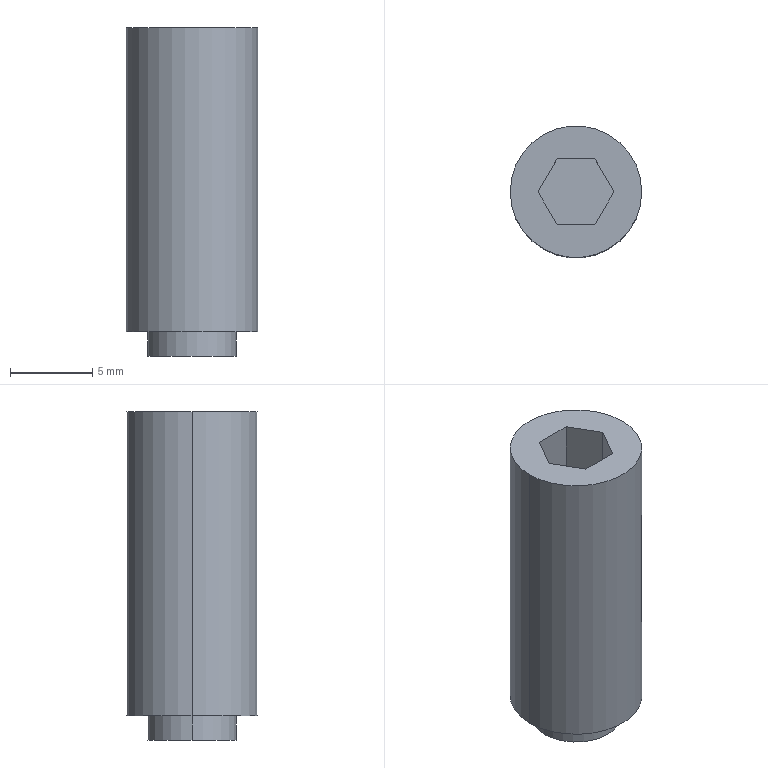Part | SolidWorks | features BaseBody 1 | 1 solid | 14 faces | box 8 x 8 x 20 mm | volume 908.839 mm3 | plane 10 | cylinder 4 | commonest cylinder face diameters 5.4 x2 8 x2
STEP:
#1=CARTESIAN_POINT('',(-2.7,0.,-1.5));
#2=VERTEX_POINT('',#1);
#3=CARTESIAN_POINT('',(2.7,0.,-1.5));
#4=VERTEX_POINT('',#3);
#5=CARTESIAN_POINT('',(0.,0.,-1.5));
#6=DIRECTION('',(0.,0.,-1.));
#7=DIRECTION('',(-1.,0.,0.));
#8=AXIS2_PLACEMENT_3D('',#5,#6,#7);
#9=CIRCLE('',#8,2.7);
#10=EDGE_CURVE('',#2,#4,#9,.T.);
#11=ORIENTED_EDGE('',*,*,#10,.T.);
#12=CARTESIAN_POINT('',(2.7,0.,-3.));
#13=VERTEX_POINT('',#12);
#14=CARTESIAN_POINT('',(2.7,0.,-3.));
#15=DIRECTION('',(0.,0.,-1.));
#16=VECTOR('',#15,1000.);
#17=LINE('',#14,#16);
#18=EDGE_CURVE('',#4,#13,#17,.T.);
#19=ORIENTED_EDGE('',*,*,#18,.T.);
#20=CARTESIAN_POINT('',(-2.7,0.,-3.));
#21=VERTEX_POINT('',#20);
#22=CARTESIAN_POINT('',(0.,0.,-3.));
#23=DIRECTION('',(0.,0.,-1.));
#24=DIRECTION('',(-1.,0.,0.));
#25=AXIS2_PLACEMENT_3D('',#22,#23,#24);
#26=CIRCLE('',#25,2.7);
#27=EDGE_CURVE('',#21,#13,#26,.T.);
#28=ORIENTED_EDGE('',*,*,#27,.F.);
#29=CARTESIAN_POINT('',(-2.7,0.,-3.));
#30=DIRECTION('',(0.,0.,-1.));
#31=VECTOR('',#30,1000.);
#32=LINE('',#29,#31);
#33=EDGE_CURVE('',#2,#21,#32,.T.);
#34=ORIENTED_EDGE('',*,*,#33,.F.);
#35=EDGE_LOOP('',(#11,#19,#28,#34));
#36=FACE_OUTER_BOUND('',#35,.T.);
#37=CARTESIAN_POINT('',(0.,0.,-3.));
#38=DIRECTION('',(0.,0.,-1.));
#39=DIRECTION('',(-1.,0.,0.));
#40=AXIS2_PLACEMENT_3D('',#37,#38,#39);
#41=CYLINDRICAL_SURFACE('',#40,2.7);
#42=ADVANCED_FACE('',(#36),#41,.T.);
#43=CARTESIAN_POINT('',(-4.,0.,17.));
#44=VERTEX_POINT('',#43);
#45=CARTESIAN_POINT('',(4.,0.,17.));
#46=VERTEX_POINT('',#45);
#47=CARTESIAN_POINT('',(0.,0.,17.));
#48=DIRECTION('',(0.,0.,-1.));
#49=DIRECTION('',(-1.,0.,0.));
#50=AXIS2_PLACEMENT_3D('',#47,#48,#49);
#51=CIRCLE('',#50,4.);
#52=EDGE_CURVE('',#44,#46,#51,.T.);
#53=ORIENTED_EDGE('',*,*,#52,.T.);
#54=CARTESIAN_POINT('',(4.,0.,-1.5));
#55=VERTEX_POINT('',#54);
#56=CARTESIAN_POINT('',(4.,0.,-3.));
#57=DIRECTION('',(0.,0.,-1.));
#58=VECTOR('',#57,1000.);
#59=LINE('',#56,#58);
#60=EDGE_CURVE('',#46,#55,#59,.T.);
#61=ORIENTED_EDGE('',*,*,#60,.T.);
#62=CARTESIAN_POINT('',(-4.,0.,-1.5));
#63=VERTEX_POINT('',#62);
#64=CARTESIAN_POINT('',(0.,0.,-1.5));
#65=DIRECTION('',(0.,0.,-1.));
#66=DIRECTION('',(-1.,0.,0.));
#67=AXIS2_PLACEMENT_3D('',#64,#65,#66);
#68=CIRCLE('',#67,4.);
#69=EDGE_CURVE('',#63,#55,#68,.T.);
#70=ORIENTED_EDGE('',*,*,#69,.F.);
#71=CARTESIAN_POINT('',(-4.,0.,-3.));
#72=DIRECTION('',(0.,0.,-1.));
#73=VECTOR('',#72,1000.);
#74=LINE('',#71,#73);
#75=EDGE_CURVE('',#44,#63,#74,.T.);
#76=ORIENTED_EDGE('',*,*,#75,.F.);
#77=EDGE_LOOP('',(#53,#61,#70,#76));
#78=FACE_OUTER_BOUND('',#77,.T.);
#79=CARTESIAN_POINT('',(0.,0.,-3.));
#80=DIRECTION('',(0.,0.,-1.));
#81=DIRECTION('',(-1.,0.,0.));
#82=AXIS2_PLACEMENT_3D('',#79,#80,#81);
#83=CYLINDRICAL_SURFACE('',#82,4.);
#84=ADVANCED_FACE('',(#78),#83,.T.);
#85=ORIENTED_EDGE('',*,*,#52,.F.);
#86=CARTESIAN_POINT('',(0.,0.,17.));
#87=DIRECTION('',(0.,0.,-1.));
#88=DIRECTION('',(-1.,0.,0.));
#89=AXIS2_PLACEMENT_3D('',#86,#87,#88);
#90=CIRCLE('',#89,4.);
#91=EDGE_CURVE('',#46,#44,#90,.T.);
#92=ORIENTED_EDGE('',*,*,#91,.F.);
#93=EDGE_LOOP('',(#85,#92));
#94=FACE_OUTER_BOUND('',#93,.T.);
#95=CARTESIAN_POINT('',(2.309,0.,17.));
#96=VERTEX_POINT('',#95);
#97=CARTESIAN_POINT('',(1.155,2.,17.));
#98=VERTEX_POINT('',#97);
#99=CARTESIAN_POINT('',(2.309,0.,17.));
#100=DIRECTION('',(-0.5,0.866,0.));
#101=VECTOR('',#100,1000.);
#102=LINE('',#99,#101);
#103=EDGE_CURVE('',#96,#98,#102,.T.);
#104=ORIENTED_EDGE('',*,*,#103,.F.);
#105=CARTESIAN_POINT('',(1.155,-2.,17.));
#106=VERTEX_POINT('',#105);
#107=CARTESIAN_POINT('',(1.155,-2.,17.));
#108=DIRECTION('',(0.5,0.866,0.));
#109=VECTOR('',#108,1000.);
#110=LINE('',#107,#109);
#111=EDGE_CURVE('',#106,#96,#110,.T.);
#112=ORIENTED_EDGE('',*,*,#111,.F.);
#113=CARTESIAN_POINT('',(-1.155,-2.,17.));
#114=VERTEX_POINT('',#113);
#115=CARTESIAN_POINT('',(-1.155,-2.,17.));
#116=DIRECTION('',(1.,0.,0.));
#117=VECTOR('',#116,1000.);
#118=LINE('',#115,#117);
#119=EDGE_CURVE('',#114,#106,#118,.T.);
#120=ORIENTED_EDGE('',*,*,#119,.F.);
#121=CARTESIAN_POINT('',(-2.309,0.,17.));
#122=VERTEX_POINT('',#121);
#123=CARTESIAN_POINT('',(-2.309,0.,17.));
#124=DIRECTION('',(0.5,-0.866,0.));
#125=VECTOR('',#124,1000.);
#126=LINE('',#123,#125);
#127=EDGE_CURVE('',#122,#114,#126,.T.);
#128=ORIENTED_EDGE('',*,*,#127,.F.);
#129=CARTESIAN_POINT('',(-1.155,2.,17.));
#130=VERTEX_POINT('',#129);
#131=CARTESIAN_POINT('',(-1.155,2.,17.));
#132=DIRECTION('',(-0.5,-0.866,0.));
#133=VECTOR('',#132,1000.);
#134=LINE('',#131,#133);
#135=EDGE_CURVE('',#130,#122,#134,.T.);
#136=ORIENTED_EDGE('',*,*,#135,.F.);
#137=CARTESIAN_POINT('',(-1.155,2.,17.));
#138=DIRECTION('',(1.,0.,0.));
#139=VECTOR('',#138,1000.);
#140=LINE('',#137,#139);
#141=EDGE_CURVE('',#130,#98,#140,.T.);
#142=ORIENTED_EDGE('',*,*,#141,.T.);
#143=EDGE_LOOP('',(#104,#112,#120,#128,#136,#142));
#144=FACE_BOUND('',#143,.T.);
#145=CARTESIAN_POINT('',(0.,0.,17.));
#146=DIRECTION('',(0.,0.,-1.));
#147=DIRECTION('',(-1.,0.,0.));
#148=AXIS2_PLACEMENT_3D('',#145,#146,#147);
#149=PLANE('',#148);
#150=ADVANCED_FACE('',(#94,#144),#149,.F.);
#151=ORIENTED_EDGE('',*,*,#60,.F.);
#152=ORIENTED_EDGE('',*,*,#91,.T.);
#153=ORIENTED_EDGE('',*,*,#75,.T.);
#154=CARTESIAN_POINT('',(0.,0.,-1.5));
#155=DIRECTION('',(0.,0.,-1.));
#156=DIRECTION('',(-1.,0.,0.));
#157=AXIS2_PLACEMENT_3D('',#154,#155,#156);
#158=CIRCLE('',#157,4.);
#159=EDGE_CURVE('',#55,#63,#158,.T.);
#160=ORIENTED_EDGE('',*,*,#159,.F.);
#161=EDGE_LOOP('',(#151,#152,#153,#160));
#162=FACE_OUTER_BOUND('',#161,.T.);
#163=CARTESIAN_POINT('',(0.,0.,-3.));
#164=DIRECTION('',(0.,0.,-1.));
#165=DIRECTION('',(-1.,0.,0.));
#166=AXIS2_PLACEMENT_3D('',#163,#164,#165);
#167=CYLINDRICAL_SURFACE('',#166,4.);
#168=ADVANCED_FACE('',(#162),#167,.T.);
#169=ORIENTED_EDGE('',*,*,#103,.T.);
#170=CARTESIAN_POINT('',(1.155,2.,13.));
#171=VERTEX_POINT('',#170);
#172=CARTESIAN_POINT('',(1.155,2.,13.));
#173=DIRECTION('',(0.,0.,1.));
#174=VECTOR('',#173,1000.);
#175=LINE('',#172,#174);
#176=EDGE_CURVE('',#171,#98,#175,.T.);
#177=ORIENTED_EDGE('',*,*,#176,.F.);
#178=CARTESIAN_POINT('',(2.309,0.,13.));
#179=VERTEX_POINT('',#178);
#180=CARTESIAN_POINT('',(2.309,0.,13.));
#181=DIRECTION('',(-0.5,0.866,0.));
#182=VECTOR('',#181,1000.);
#183=LINE('',#180,#182);
#184=EDGE_CURVE('',#179,#171,#183,.T.);
#185=ORIENTED_EDGE('',*,*,#184,.F.);
#186=CARTESIAN_POINT('',(2.309,0.,13.));
#187=DIRECTION('',(0.,0.,1.));
#188=VECTOR('',#187,1000.);
#189=LINE('',#186,#188);
#190=EDGE_CURVE('',#179,#96,#189,.T.);
#191=ORIENTED_EDGE('',*,*,#190,.T.);
#192=EDGE_LOOP('',(#169,#177,#185,#191));
#193=FACE_OUTER_BOUND('',#192,.T.);
#194=CARTESIAN_POINT('',(2.309,0.,13.));
#195=DIRECTION('',(0.866,0.5,0.));
#196=DIRECTION('',(-0.5,0.866,0.));
#197=AXIS2_PLACEMENT_3D('',#194,#195,#196);
#198=PLANE('',#197);
#199=ADVANCED_FACE('',(#193),#198,.F.);
#200=ORIENTED_EDGE('',*,*,#111,.T.);
#201=ORIENTED_EDGE('',*,*,#190,.F.);
#202=CARTESIAN_POINT('',(1.155,-2.,13.));
#203=VERTEX_POINT('',#202);
#204=CARTESIAN_POINT('',(1.155,-2.,13.));
#205=DIRECTION('',(0.5,0.866,0.));
#206=VECTOR('',#205,1000.);
#207=LINE('',#204,#206);
#208=EDGE_CURVE('',#203,#179,#207,.T.);
#209=ORIENTED_EDGE('',*,*,#208,.F.);
#210=CARTESIAN_POINT('',(1.155,-2.,13.));
#211=DIRECTION('',(0.,0.,1.));
#212=VECTOR('',#211,1000.);
#213=LINE('',#210,#212);
#214=EDGE_CURVE('',#203,#106,#213,.T.);
#215=ORIENTED_EDGE('',*,*,#214,.T.);
#216=EDGE_LOOP('',(#200,#201,#209,#215));
#217=FACE_OUTER_BOUND('',#216,.T.);
#218=CARTESIAN_POINT('',(1.155,-2.,13.));
#219=DIRECTION('',(0.866,-0.5,0.));
#220=DIRECTION('',(0.5,0.866,0.));
#221=AXIS2_PLACEMENT_3D('',#218,#219,#220);
#222=PLANE('',#221);
#223=ADVANCED_FACE('',(#217),#222,.F.);
#224=ORIENTED_EDGE('',*,*,#119,.T.);
#225=ORIENTED_EDGE('',*,*,#214,.F.);
#226=CARTESIAN_POINT('',(-1.155,-2.,13.));
#227=VERTEX_POINT('',#226);
#228=CARTESIAN_POINT('',(-1.155,-2.,13.));
#229=DIRECTION('',(1.,0.,0.));
#230=VECTOR('',#229,1000.);
#231=LINE('',#228,#230);
#232=EDGE_CURVE('',#227,#203,#231,.T.);
#233=ORIENTED_EDGE('',*,*,#232,.F.);
#234=CARTESIAN_POINT('',(-1.155,-2.,13.));
#235=DIRECTION('',(0.,0.,1.));
#236=VECTOR('',#235,1000.);
#237=LINE('',#234,#236);
#238=EDGE_CURVE('',#227,#114,#237,.T.);
#239=ORIENTED_EDGE('',*,*,#238,.T.);
#240=EDGE_LOOP('',(#224,#225,#233,#239));
#241=FACE_OUTER_BOUND('',#240,.T.);
#242=CARTESIAN_POINT('',(-1.155,-2.,13.));
#243=DIRECTION('',(0.,-1.,0.));
#244=DIRECTION('',(0.,0.,-1.));
#245=AXIS2_PLACEMENT_3D('',#242,#243,#244);
#246=PLANE('',#245);
#247=ADVANCED_FACE('',(#241),#246,.F.);
#248=ORIENTED_EDGE('',*,*,#127,.T.);
#249=ORIENTED_EDGE('',*,*,#238,.F.);
#250=CARTESIAN_POINT('',(-2.309,0.,13.));
#251=VERTEX_POINT('',#250);
#252=CARTESIAN_POINT('',(-2.309,0.,13.));
#253=DIRECTION('',(0.5,-0.866,0.));
#254=VECTOR('',#253,1000.);
#255=LINE('',#252,#254);
#256=EDGE_CURVE('',#251,#227,#255,.T.);
#257=ORIENTED_EDGE('',*,*,#256,.F.);
#258=CARTESIAN_POINT('',(-2.309,0.,13.));
#259=DIRECTION('',(0.,0.,1.));
#260=VECTOR('',#259,1000.);
#261=LINE('',#258,#260);
#262=EDGE_CURVE('',#251,#122,#261,.T.);
#263=ORIENTED_EDGE('',*,*,#262,.T.);
#264=EDGE_LOOP('',(#248,#249,#257,#263));
#265=FACE_OUTER_BOUND('',#264,.T.);
#266=CARTESIAN_POINT('',(-2.309,0.,13.));
#267=DIRECTION('',(-0.866,-0.5,0.));
#268=DIRECTION('',(0.5,-0.866,0.));
#269=AXIS2_PLACEMENT_3D('',#266,#267,#268);
#270=PLANE('',#269);
#271=ADVANCED_FACE('',(#265),#270,.F.);
#272=ORIENTED_EDGE('',*,*,#135,.T.);
#273=ORIENTED_EDGE('',*,*,#262,.F.);
#274=CARTESIAN_POINT('',(-1.155,2.,13.));
#275=VERTEX_POINT('',#274);
#276=CARTESIAN_POINT('',(-1.155,2.,13.));
#277=DIRECTION('',(-0.5,-0.866,0.));
#278=VECTOR('',#277,1000.);
#279=LINE('',#276,#278);
#280=EDGE_CURVE('',#275,#251,#279,.T.);
#281=ORIENTED_EDGE('',*,*,#280,.F.);
#282=CARTESIAN_POINT('',(-1.155,2.,13.));
#283=DIRECTION('',(0.,0.,1.));
#284=VECTOR('',#283,1000.);
#285=LINE('',#282,#284);
#286=EDGE_CURVE('',#275,#130,#285,.T.);
#287=ORIENTED_EDGE('',*,*,#286,.T.);
#288=EDGE_LOOP('',(#272,#273,#281,#287));
#289=FACE_OUTER_BOUND('',#288,.T.);
#290=CARTESIAN_POINT('',(-1.155,2.,13.));
#291=DIRECTION('',(-0.866,0.5,0.));
#292=DIRECTION('',(-0.5,-0.866,0.));
#293=AXIS2_PLACEMENT_3D('',#290,#291,#292);
#294=PLANE('',#293);
#295=ADVANCED_FACE('',(#289),#294,.F.);
#296=ORIENTED_EDGE('',*,*,#176,.T.);
#297=ORIENTED_EDGE('',*,*,#141,.F.);
#298=ORIENTED_EDGE('',*,*,#286,.F.);
#299=CARTESIAN_POINT('',(1.155,2.,13.));
#300=DIRECTION('',(-1.,0.,0.));
#301=VECTOR('',#300,1000.);
#302=LINE('',#299,#301);
#303=EDGE_CURVE('',#171,#275,#302,.T.);
#304=ORIENTED_EDGE('',*,*,#303,.F.);
#305=EDGE_LOOP('',(#296,#297,#298,#304));
#306=FACE_OUTER_BOUND('',#305,.T.);
#307=CARTESIAN_POINT('',(1.155,2.,13.));
#308=DIRECTION('',(0.,1.,0.));
#309=DIRECTION('',(0.,0.,1.));
#310=AXIS2_PLACEMENT_3D('',#307,#308,#309);
#311=PLANE('',#310);
#312=ADVANCED_FACE('',(#306),#311,.F.);
#313=ORIENTED_EDGE('',*,*,#10,.F.);
#314=CARTESIAN_POINT('',(0.,0.,-1.5));
#315=DIRECTION('',(0.,0.,-1.));
#316=DIRECTION('',(-1.,0.,0.));
#317=AXIS2_PLACEMENT_3D('',#314,#315,#316);
#318=CIRCLE('',#317,2.7);
#319=EDGE_CURVE('',#4,#2,#318,.T.);
#320=ORIENTED_EDGE('',*,*,#319,.F.);
#321=EDGE_LOOP('',(#313,#320));
#322=FACE_BOUND('',#321,.T.);
#323=ORIENTED_EDGE('',*,*,#69,.T.);
#324=ORIENTED_EDGE('',*,*,#159,.T.);
#325=EDGE_LOOP('',(#323,#324));
#326=FACE_OUTER_BOUND('',#325,.T.);
#327=CARTESIAN_POINT('',(0.,4.,-1.5));
#328=DIRECTION('',(0.,0.,1.));
#329=DIRECTION('',(1.,0.,0.));
#330=AXIS2_PLACEMENT_3D('',#327,#328,#329);
#331=PLANE('',#330);
#332=ADVANCED_FACE('',(#322,#326),#331,.F.);
#333=ORIENTED_EDGE('',*,*,#232,.T.);
#334=ORIENTED_EDGE('',*,*,#208,.T.);
#335=ORIENTED_EDGE('',*,*,#184,.T.);
#336=ORIENTED_EDGE('',*,*,#303,.T.);
#337=ORIENTED_EDGE('',*,*,#280,.T.);
#338=ORIENTED_EDGE('',*,*,#256,.T.);
#339=EDGE_LOOP('',(#333,#334,#335,#336,#337,#338));
#340=FACE_OUTER_BOUND('',#339,.T.);
#341=CARTESIAN_POINT('',(0.,0.,13.));
#342=DIRECTION('',(0.,0.,1.));
#343=DIRECTION('',(1.,0.,0.));
#344=AXIS2_PLACEMENT_3D('',#341,#342,#343);
#345=PLANE('',#344);
#346=ADVANCED_FACE('',(#340),#345,.T.);
#347=ORIENTED_EDGE('',*,*,#18,.F.);
#348=ORIENTED_EDGE('',*,*,#319,.T.);
#349=ORIENTED_EDGE('',*,*,#33,.T.);
#350=CARTESIAN_POINT('',(0.,0.,-3.));
#351=DIRECTION('',(0.,0.,-1.));
#352=DIRECTION('',(-1.,0.,0.));
#353=AXIS2_PLACEMENT_3D('',#350,#351,#352);
#354=CIRCLE('',#353,2.7);
#355=EDGE_CURVE('',#13,#21,#354,.T.);
#356=ORIENTED_EDGE('',*,*,#355,.F.);
#357=EDGE_LOOP('',(#347,#348,#349,#356));
#358=FACE_OUTER_BOUND('',#357,.T.);
#359=CARTESIAN_POINT('',(0.,0.,-3.));
#360=DIRECTION('',(0.,0.,-1.));
#361=DIRECTION('',(-1.,0.,0.));
#362=AXIS2_PLACEMENT_3D('',#359,#360,#361);
#363=CYLINDRICAL_SURFACE('',#362,2.7);
#364=ADVANCED_FACE('',(#358),#363,.T.);
#365=ORIENTED_EDGE('',*,*,#27,.T.);
#366=ORIENTED_EDGE('',*,*,#355,.T.);
#367=EDGE_LOOP('',(#365,#366));
#368=FACE_OUTER_BOUND('',#367,.T.);
#369=CARTESIAN_POINT('',(0.,2.7,-3.));
#370=DIRECTION('',(0.,0.,1.));
#371=DIRECTION('',(1.,0.,0.));
#372=AXIS2_PLACEMENT_3D('',#369,#370,#371);
#373=PLANE('',#372);
#374=ADVANCED_FACE('',(#368),#373,.F.);
#375=CLOSED_SHELL('',(#42,#84,#150,#168,#199,#223,#247,#271,#295,#312,#332,#346,#364,#374));
#376=MANIFOLD_SOLID_BREP('',#375);
#377=CARTESIAN_POINT('',(0.,0.,0.));
#378=DIRECTION('',(0.,0.,1.));
#379=DIRECTION('',(1.,0.,0.));
#380=AXIS2_PLACEMENT_3D('',#377,#378,#379);
#381=(LENGTH_UNIT()NAMED_UNIT(*)SI_UNIT(.MILLI.,.METRE.));
#382=UNCERTAINTY_MEASURE_WITH_UNIT(LENGTH_MEASURE(0.00001),#381,'','');
#383=(NAMED_UNIT(*)PLANE_ANGLE_UNIT()SI_UNIT($,.RADIAN.));
#384=(NAMED_UNIT(*)SI_UNIT($,.STERADIAN.)SOLID_ANGLE_UNIT());
#385=(GEOMETRIC_REPRESENTATION_CONTEXT(3)GLOBAL_UNCERTAINTY_ASSIGNED_CONTEXT((#382))GLOBAL_UNIT_ASSIGNED_CONTEXT((#381,#383,#384))REPRESENTATION_CONTEXT('',''));
#386=ADVANCED_BREP_SHAPE_REPRESENTATION('',(#376,#380),#385);